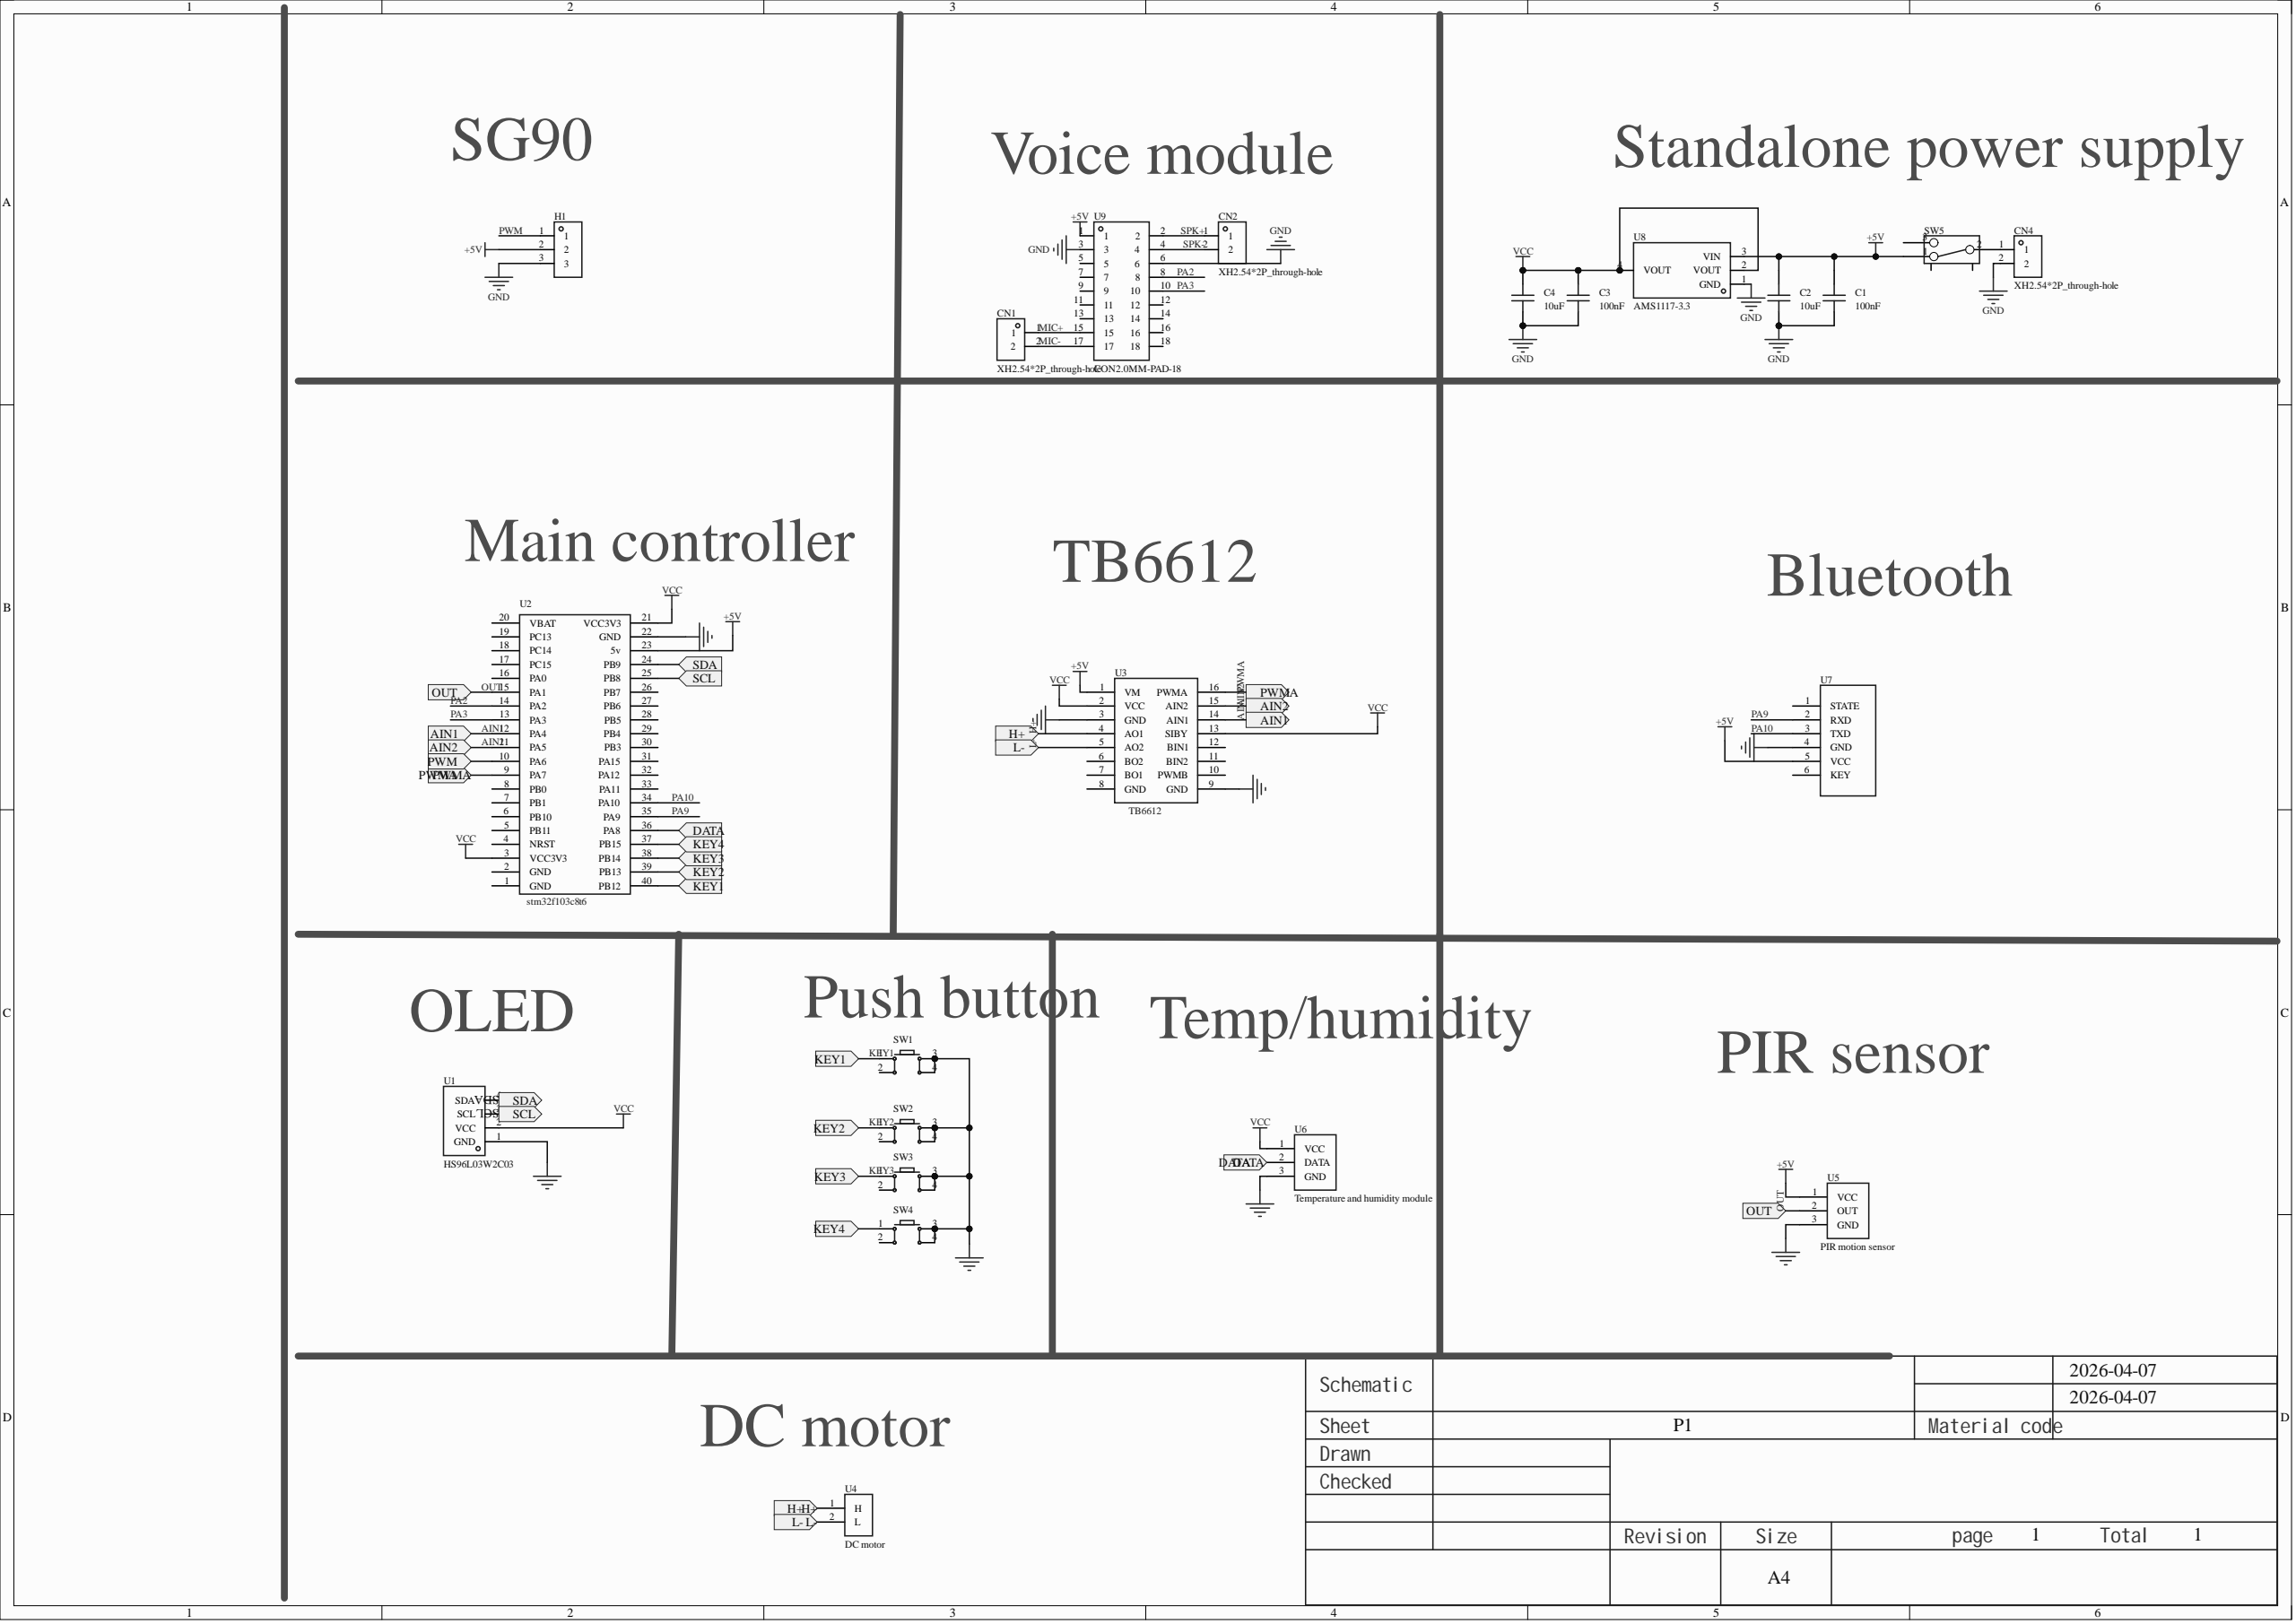Circuit board | Altium Designer | 22 parts | 25 nets
Bill of materials:
Comment,Description,Designator,Footprint,LibRef,Quantity
"100nF","","C1, C3","C0603","CAP_0603","2"
"10uF","","C2, C4","C0603","CAP_0603","2"
"XH2.54*2P_through-hole","","CN1, CN2, CN4","CONN-TH_2P-P2.50-XH2.54-2P","XH2.54*2P_直插","3"
"","","H1","HDR-TH_3P-P2.54-V-F","HDR-F_2.54_1x3P","1"
"","","SW1, SW2, SW3, SW4","按键","Key_SMD_6x6x6.5","4"
"","","SW5","拨动开关","拨动开关_正","1"
"HS96L03W2C03","Main controller: SSD1315; interface: I2C; size (inch): 0.96; resolution: 128x64;","U1","OLED-TH_L27.8-W27.2-P2.54_C9900033791","HS96L03W2C03","1"
"","","U2","STM32","stm32f103c8t6","1"
"","","U3","电机驱动模块","TB6612","1"
"","","U4","直流电机","直流电机","1"
"","","U5","人体红外模块","人体红外传感器","1"
"","","U6","DHT11温湿度","温湿度模块","1"
"","","U7","蓝牙HC-08","蓝牙HC-08","1"
"AMS1117-3.3","Output type: fixed; operating voltage: 15V; output voltage: 3.3V; output current: 1A; PSRR: 72dB@(120Hz); output polarity: positive;","U8","SOT-223-3_L6.5-W3.4-P2.30-LS7.0-BR","AMS1117-3.3_C6186","1"
"CON2.0MM-PAD-18","","U9","CONN-TH_18P-P2.00_C9900078766","CON2.0MM-PAD-18","1"
Netlist (Protel format):
[
C1
C0603
100nF



]
[
C2
C0603
10uF



]
[
C3
C0603
100nF



]
[
C4
C0603
10uF



]
[
CN1
CONN-TH_2P-P2.50-XH2.54-2P
XH2.54*2P_through-hole



]
[
CN2
CONN-TH_2P-P2.50-XH2.54-2P
XH2.54*2P_through-hole



]
[
CN4
CONN-TH_2P-P2.50-XH2.54-2P
XH2.54*2P_through-hole



]
[
H1
HDR-TH_3P-P2.54-V-F




]
[
SW1
按键




]
[
SW2
按键




]
[
SW3
按键




]
[
SW4
按键




]
[
SW5
拨动开关




]
[
U1
OLED-TH_L27.8-W27.2-P2.54_C9900033791
HS96L03W2C03



]
[
U2
STM32




]
[
U3
电机驱动模块




]
[
U4
直流电机




]
[
U5
人体红外模块




]
[
U6
DHT11温湿度




]
[
U7
蓝牙HC-08




]
[
U8
SOT-223-3_L6.5-W3.4-P2.30-LS7.0-BR
AMS1117-3.3



]
[
U9
CONN-TH_18P-P2.00_C9900078766
CON2.0MM-PAD-18



]
(
VCC
C3-2
C4-2
U1-2
U2-3
U2-21
U3-2
U3-13
U6-1
U8-2
U8-4
)
(
SPK-
CN2-2
U9-4
)
(
SPK+
CN2-1
U9-2
)
(
SDA
U1-4
U2-24
)
(
SCL
U1-3
U2-25
)
(
PWMA
U2-9
U3-16
)
(
PA10
U2-34
U7-3
)
(
PA9
U2-35
U7-2
)
(
PA3
U2-13
U9-10
)
(
PA2
U2-14
U9-8
)
(
OUT
U2-15
U5-2
)
(
NetSW4_1
SW4-1
U2-37
)
(
NetCN4_1
CN4-1
SW5-2
)
(
MIC-
CN1-2
U9-17
)
(
MIC+
CN1-1
U9-15
)
(
L-
U3-5
U4-2
)
(
KEY3
SW3-1
U2-38
)
(
KEY2
SW2-1
U2-39
)
(
KEY1
SW1-1
U2-40
)
(
H+
U3-4
U4-1
)
(
GND
C1-1
C2-1
C3-1
C4-1
CN4-2
H1-3
SW1-3
SW1-4
SW2-3
SW2-4
SW3-3
SW3-4
SW4-3
SW4-4
U1-1
U2-22
U3-3
U3-9
U5-3
U6-3
U7-4
U8-1
U9-3
U9-6
)
(
DATA
U2-36
U6-2
)
(
AIN2
U2-11
U3-15
)
(
AIN1
U2-12
U3-14
)
(
+5V
C1-2
C2-2
H1-2
SW5-1
U2-23
U3-1
U5-1
U7-5
U8-3
U9-1
)